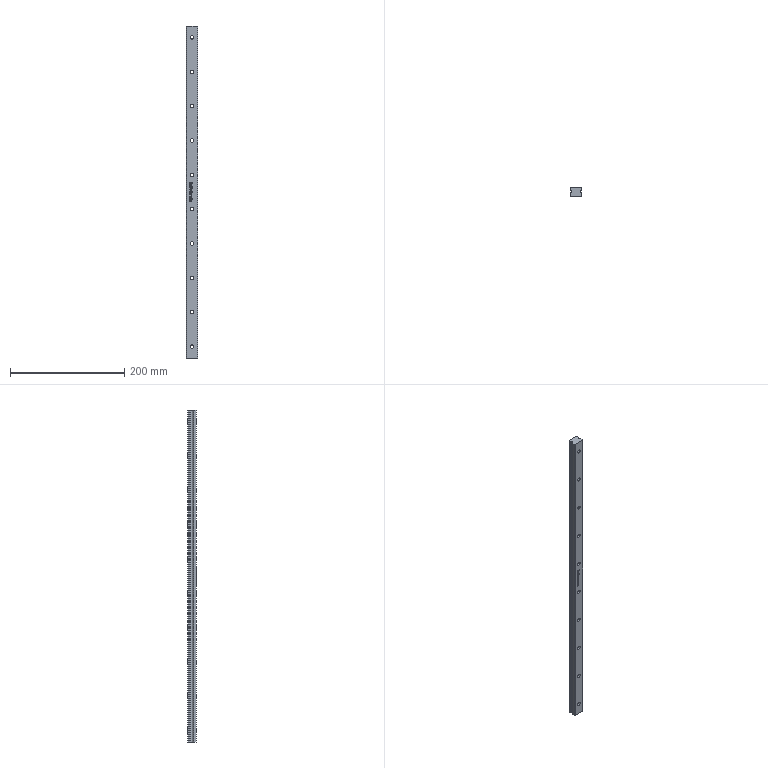Part | STEP file | EGH20CA2R580Z0C,E=20MM | 1 solid | 210 faces | box 20 x 15.5 x 580 mm | volume 158003 mm3 | plane 107 | spline 56 | cylinder 47 | commonest cylinder face diameters 6 x20 9.5 x20 4.2 x4 5 x3